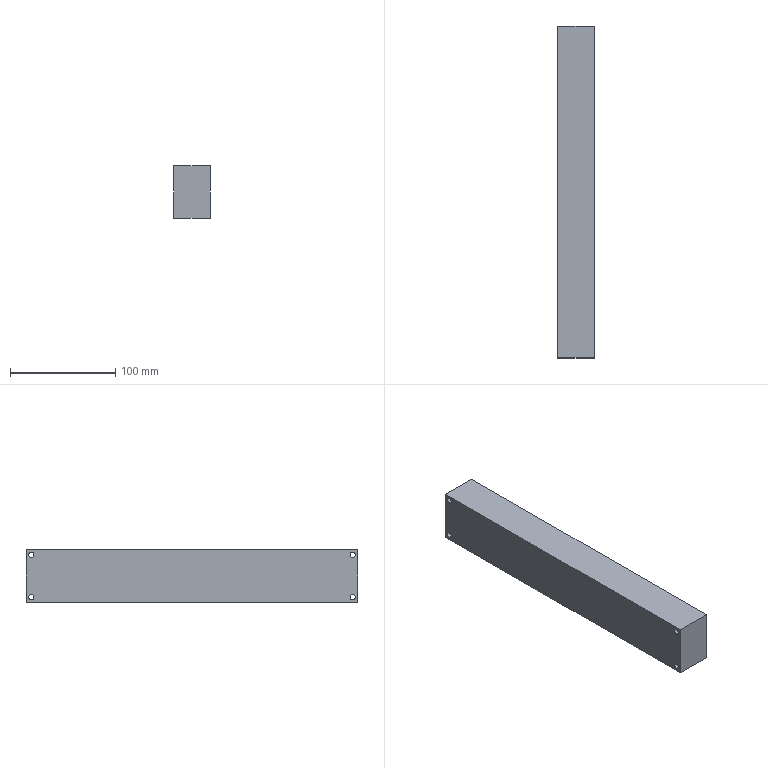Part | SolidWorks | features Extrusion 1, ICE 1 | 1 solid | 14 faces | box 35 x 315 x 50 mm | volume 548501 mm3 | cylinder 8 | plane 6 | commonest cylinder face diameters 5 x8
STEP:
#1=CARTESIAN_POINT('',(35.,5.,2.5));
#2=VERTEX_POINT('',#1);
#3=CARTESIAN_POINT('',(35.,5.,7.5));
#4=VERTEX_POINT('',#3);
#5=CARTESIAN_POINT('',(35.,5.,5.));
#6=DIRECTION('',(-1.,0.,0.));
#7=DIRECTION('',(0.,0.,1.));
#8=AXIS2_PLACEMENT_3D('',#5,#6,#7);
#9=CIRCLE('',#8,2.5);
#10=EDGE_CURVE('',#2,#4,#9,.T.);
#11=ORIENTED_EDGE('',*,*,#10,.F.);
#12=CARTESIAN_POINT('',(0.,5.,2.5));
#13=VERTEX_POINT('',#12);
#14=CARTESIAN_POINT('',(40.,5.,2.5));
#15=DIRECTION('',(-1.,0.,0.));
#16=VECTOR('',#15,1000.);
#17=LINE('',#14,#16);
#18=EDGE_CURVE('',#2,#13,#17,.T.);
#19=ORIENTED_EDGE('',*,*,#18,.T.);
#20=CARTESIAN_POINT('',(0.,5.,7.5));
#21=VERTEX_POINT('',#20);
#22=CARTESIAN_POINT('',(0.,5.,5.));
#23=DIRECTION('',(-1.,0.,0.));
#24=DIRECTION('',(0.,0.,1.));
#25=AXIS2_PLACEMENT_3D('',#22,#23,#24);
#26=CIRCLE('',#25,2.5);
#27=EDGE_CURVE('',#13,#21,#26,.T.);
#28=ORIENTED_EDGE('',*,*,#27,.T.);
#29=CARTESIAN_POINT('',(40.,5.,7.5));
#30=DIRECTION('',(-1.,0.,0.));
#31=VECTOR('',#30,1000.);
#32=LINE('',#29,#31);
#33=EDGE_CURVE('',#4,#21,#32,.T.);
#34=ORIENTED_EDGE('',*,*,#33,.F.);
#35=EDGE_LOOP('',(#11,#19,#28,#34));
#36=FACE_OUTER_BOUND('',#35,.T.);
#37=CARTESIAN_POINT('',(40.,5.,5.));
#38=DIRECTION('',(-1.,0.,0.));
#39=DIRECTION('',(0.,0.,1.));
#40=AXIS2_PLACEMENT_3D('',#37,#38,#39);
#41=CYLINDRICAL_SURFACE('',#40,2.5);
#42=ADVANCED_FACE('',(#36),#41,.F.);
#43=CARTESIAN_POINT('',(35.,5.,42.5));
#44=VERTEX_POINT('',#43);
#45=CARTESIAN_POINT('',(35.,5.,47.5));
#46=VERTEX_POINT('',#45);
#47=CARTESIAN_POINT('',(35.,5.,45.));
#48=DIRECTION('',(-1.,0.,0.));
#49=DIRECTION('',(0.,0.,1.));
#50=AXIS2_PLACEMENT_3D('',#47,#48,#49);
#51=CIRCLE('',#50,2.5);
#52=EDGE_CURVE('',#44,#46,#51,.T.);
#53=ORIENTED_EDGE('',*,*,#52,.F.);
#54=CARTESIAN_POINT('',(0.,5.,42.5));
#55=VERTEX_POINT('',#54);
#56=CARTESIAN_POINT('',(40.,5.,42.5));
#57=DIRECTION('',(-1.,0.,0.));
#58=VECTOR('',#57,1000.);
#59=LINE('',#56,#58);
#60=EDGE_CURVE('',#44,#55,#59,.T.);
#61=ORIENTED_EDGE('',*,*,#60,.T.);
#62=CARTESIAN_POINT('',(0.,5.,47.5));
#63=VERTEX_POINT('',#62);
#64=CARTESIAN_POINT('',(0.,5.,45.));
#65=DIRECTION('',(-1.,0.,0.));
#66=DIRECTION('',(0.,0.,1.));
#67=AXIS2_PLACEMENT_3D('',#64,#65,#66);
#68=CIRCLE('',#67,2.5);
#69=EDGE_CURVE('',#55,#63,#68,.T.);
#70=ORIENTED_EDGE('',*,*,#69,.T.);
#71=CARTESIAN_POINT('',(40.,5.,47.5));
#72=DIRECTION('',(-1.,0.,0.));
#73=VECTOR('',#72,1000.);
#74=LINE('',#71,#73);
#75=EDGE_CURVE('',#46,#63,#74,.T.);
#76=ORIENTED_EDGE('',*,*,#75,.F.);
#77=EDGE_LOOP('',(#53,#61,#70,#76));
#78=FACE_OUTER_BOUND('',#77,.T.);
#79=CARTESIAN_POINT('',(40.,5.,45.));
#80=DIRECTION('',(-1.,0.,0.));
#81=DIRECTION('',(0.,0.,1.));
#82=AXIS2_PLACEMENT_3D('',#79,#80,#81);
#83=CYLINDRICAL_SURFACE('',#82,2.5);
#84=ADVANCED_FACE('',(#78),#83,.F.);
#85=CARTESIAN_POINT('',(35.,310.,2.5));
#86=VERTEX_POINT('',#85);
#87=CARTESIAN_POINT('',(35.,310.,7.5));
#88=VERTEX_POINT('',#87);
#89=CARTESIAN_POINT('',(35.,310.,5.));
#90=DIRECTION('',(-1.,0.,0.));
#91=DIRECTION('',(0.,0.,1.));
#92=AXIS2_PLACEMENT_3D('',#89,#90,#91);
#93=CIRCLE('',#92,2.5);
#94=EDGE_CURVE('',#86,#88,#93,.T.);
#95=ORIENTED_EDGE('',*,*,#94,.F.);
#96=CARTESIAN_POINT('',(0.,310.,2.5));
#97=VERTEX_POINT('',#96);
#98=CARTESIAN_POINT('',(40.,310.,2.5));
#99=DIRECTION('',(-1.,0.,0.));
#100=VECTOR('',#99,1000.);
#101=LINE('',#98,#100);
#102=EDGE_CURVE('',#86,#97,#101,.T.);
#103=ORIENTED_EDGE('',*,*,#102,.T.);
#104=CARTESIAN_POINT('',(0.,310.,7.5));
#105=VERTEX_POINT('',#104);
#106=CARTESIAN_POINT('',(0.,310.,5.));
#107=DIRECTION('',(-1.,0.,0.));
#108=DIRECTION('',(0.,0.,1.));
#109=AXIS2_PLACEMENT_3D('',#106,#107,#108);
#110=CIRCLE('',#109,2.5);
#111=EDGE_CURVE('',#97,#105,#110,.T.);
#112=ORIENTED_EDGE('',*,*,#111,.T.);
#113=CARTESIAN_POINT('',(40.,310.,7.5));
#114=DIRECTION('',(-1.,0.,0.));
#115=VECTOR('',#114,1000.);
#116=LINE('',#113,#115);
#117=EDGE_CURVE('',#88,#105,#116,.T.);
#118=ORIENTED_EDGE('',*,*,#117,.F.);
#119=EDGE_LOOP('',(#95,#103,#112,#118));
#120=FACE_OUTER_BOUND('',#119,.T.);
#121=CARTESIAN_POINT('',(40.,310.,5.));
#122=DIRECTION('',(-1.,0.,0.));
#123=DIRECTION('',(0.,0.,1.));
#124=AXIS2_PLACEMENT_3D('',#121,#122,#123);
#125=CYLINDRICAL_SURFACE('',#124,2.5);
#126=ADVANCED_FACE('',(#120),#125,.F.);
#127=CARTESIAN_POINT('',(35.,310.,42.5));
#128=VERTEX_POINT('',#127);
#129=CARTESIAN_POINT('',(35.,310.,47.5));
#130=VERTEX_POINT('',#129);
#131=CARTESIAN_POINT('',(35.,310.,45.));
#132=DIRECTION('',(-1.,0.,0.));
#133=DIRECTION('',(0.,0.,1.));
#134=AXIS2_PLACEMENT_3D('',#131,#132,#133);
#135=CIRCLE('',#134,2.5);
#136=EDGE_CURVE('',#128,#130,#135,.T.);
#137=ORIENTED_EDGE('',*,*,#136,.F.);
#138=CARTESIAN_POINT('',(0.,310.,42.5));
#139=VERTEX_POINT('',#138);
#140=CARTESIAN_POINT('',(40.,310.,42.5));
#141=DIRECTION('',(-1.,0.,0.));
#142=VECTOR('',#141,1000.);
#143=LINE('',#140,#142);
#144=EDGE_CURVE('',#128,#139,#143,.T.);
#145=ORIENTED_EDGE('',*,*,#144,.T.);
#146=CARTESIAN_POINT('',(0.,310.,47.5));
#147=VERTEX_POINT('',#146);
#148=CARTESIAN_POINT('',(0.,310.,45.));
#149=DIRECTION('',(-1.,0.,0.));
#150=DIRECTION('',(0.,0.,1.));
#151=AXIS2_PLACEMENT_3D('',#148,#149,#150);
#152=CIRCLE('',#151,2.5);
#153=EDGE_CURVE('',#139,#147,#152,.T.);
#154=ORIENTED_EDGE('',*,*,#153,.T.);
#155=CARTESIAN_POINT('',(40.,310.,47.5));
#156=DIRECTION('',(-1.,0.,0.));
#157=VECTOR('',#156,1000.);
#158=LINE('',#155,#157);
#159=EDGE_CURVE('',#130,#147,#158,.T.);
#160=ORIENTED_EDGE('',*,*,#159,.F.);
#161=EDGE_LOOP('',(#137,#145,#154,#160));
#162=FACE_OUTER_BOUND('',#161,.T.);
#163=CARTESIAN_POINT('',(40.,310.,45.));
#164=DIRECTION('',(-1.,0.,0.));
#165=DIRECTION('',(0.,0.,1.));
#166=AXIS2_PLACEMENT_3D('',#163,#164,#165);
#167=CYLINDRICAL_SURFACE('',#166,2.5);
#168=ADVANCED_FACE('',(#162),#167,.F.);
#169=CARTESIAN_POINT('',(0.,5.,5.));
#170=DIRECTION('',(-1.,0.,0.));
#171=DIRECTION('',(0.,0.,1.));
#172=AXIS2_PLACEMENT_3D('',#169,#170,#171);
#173=CIRCLE('',#172,2.5);
#174=EDGE_CURVE('',#21,#13,#173,.T.);
#175=ORIENTED_EDGE('',*,*,#174,.F.);
#176=ORIENTED_EDGE('',*,*,#27,.F.);
#177=EDGE_LOOP('',(#175,#176));
#178=FACE_BOUND('',#177,.T.);
#179=CARTESIAN_POINT('',(0.,5.,45.));
#180=DIRECTION('',(-1.,0.,0.));
#181=DIRECTION('',(0.,0.,1.));
#182=AXIS2_PLACEMENT_3D('',#179,#180,#181);
#183=CIRCLE('',#182,2.5);
#184=EDGE_CURVE('',#63,#55,#183,.T.);
#185=ORIENTED_EDGE('',*,*,#184,.F.);
#186=ORIENTED_EDGE('',*,*,#69,.F.);
#187=EDGE_LOOP('',(#185,#186));
#188=FACE_BOUND('',#187,.T.);
#189=CARTESIAN_POINT('',(0.,310.,5.));
#190=DIRECTION('',(-1.,0.,0.));
#191=DIRECTION('',(0.,0.,1.));
#192=AXIS2_PLACEMENT_3D('',#189,#190,#191);
#193=CIRCLE('',#192,2.5);
#194=EDGE_CURVE('',#105,#97,#193,.T.);
#195=ORIENTED_EDGE('',*,*,#194,.F.);
#196=ORIENTED_EDGE('',*,*,#111,.F.);
#197=EDGE_LOOP('',(#195,#196));
#198=FACE_BOUND('',#197,.T.);
#199=CARTESIAN_POINT('',(0.,310.,45.));
#200=DIRECTION('',(-1.,0.,0.));
#201=DIRECTION('',(0.,0.,1.));
#202=AXIS2_PLACEMENT_3D('',#199,#200,#201);
#203=CIRCLE('',#202,2.5);
#204=EDGE_CURVE('',#147,#139,#203,.T.);
#205=ORIENTED_EDGE('',*,*,#204,.F.);
#206=ORIENTED_EDGE('',*,*,#153,.F.);
#207=EDGE_LOOP('',(#205,#206));
#208=FACE_BOUND('',#207,.T.);
#209=CARTESIAN_POINT('',(0.,315.,0.));
#210=VERTEX_POINT('',#209);
#211=CARTESIAN_POINT('',(0.,0.,0.));
#212=VERTEX_POINT('',#211);
#213=CARTESIAN_POINT('',(0.,0.,0.));
#214=DIRECTION('',(0.,-1.,0.));
#215=VECTOR('',#214,1000.);
#216=LINE('',#213,#215);
#217=EDGE_CURVE('',#210,#212,#216,.T.);
#218=ORIENTED_EDGE('',*,*,#217,.T.);
#219=CARTESIAN_POINT('',(0.,0.,50.));
#220=VERTEX_POINT('',#219);
#221=CARTESIAN_POINT('',(0.,0.,50.));
#222=DIRECTION('',(0.,0.,-1.));
#223=VECTOR('',#222,1000.);
#224=LINE('',#221,#223);
#225=EDGE_CURVE('',#220,#212,#224,.T.);
#226=ORIENTED_EDGE('',*,*,#225,.F.);
#227=CARTESIAN_POINT('',(0.,315.,50.));
#228=VERTEX_POINT('',#227);
#229=CARTESIAN_POINT('',(0.,0.,50.));
#230=DIRECTION('',(0.,-1.,0.));
#231=VECTOR('',#230,1000.);
#232=LINE('',#229,#231);
#233=EDGE_CURVE('',#228,#220,#232,.T.);
#234=ORIENTED_EDGE('',*,*,#233,.F.);
#235=CARTESIAN_POINT('',(0.,315.,50.));
#236=DIRECTION('',(0.,0.,-1.));
#237=VECTOR('',#236,1000.);
#238=LINE('',#235,#237);
#239=EDGE_CURVE('',#228,#210,#238,.T.);
#240=ORIENTED_EDGE('',*,*,#239,.T.);
#241=EDGE_LOOP('',(#218,#226,#234,#240));
#242=FACE_OUTER_BOUND('',#241,.T.);
#243=CARTESIAN_POINT('',(0.,0.,50.));
#244=DIRECTION('',(1.,0.,0.));
#245=DIRECTION('',(0.,0.,-1.));
#246=AXIS2_PLACEMENT_3D('',#243,#244,#245);
#247=PLANE('',#246);
#248=ADVANCED_FACE('',(#178,#188,#198,#208,#242),#247,.F.);
#249=CARTESIAN_POINT('',(35.,0.,0.));
#250=VERTEX_POINT('',#249);
#251=CARTESIAN_POINT('',(0.,0.,0.));
#252=DIRECTION('',(1.,0.,0.));
#253=VECTOR('',#252,1000.);
#254=LINE('',#251,#253);
#255=EDGE_CURVE('',#212,#250,#254,.T.);
#256=ORIENTED_EDGE('',*,*,#255,.T.);
#257=CARTESIAN_POINT('',(35.,0.,50.));
#258=VERTEX_POINT('',#257);
#259=CARTESIAN_POINT('',(35.,0.,50.));
#260=DIRECTION('',(0.,0.,-1.));
#261=VECTOR('',#260,1000.);
#262=LINE('',#259,#261);
#263=EDGE_CURVE('',#258,#250,#262,.T.);
#264=ORIENTED_EDGE('',*,*,#263,.F.);
#265=CARTESIAN_POINT('',(0.,0.,50.));
#266=DIRECTION('',(1.,0.,0.));
#267=VECTOR('',#266,1000.);
#268=LINE('',#265,#267);
#269=EDGE_CURVE('',#220,#258,#268,.T.);
#270=ORIENTED_EDGE('',*,*,#269,.F.);
#271=ORIENTED_EDGE('',*,*,#225,.T.);
#272=EDGE_LOOP('',(#256,#264,#270,#271));
#273=FACE_OUTER_BOUND('',#272,.T.);
#274=CARTESIAN_POINT('',(0.,0.,50.));
#275=DIRECTION('',(0.,1.,0.));
#276=DIRECTION('',(0.,0.,1.));
#277=AXIS2_PLACEMENT_3D('',#274,#275,#276);
#278=PLANE('',#277);
#279=ADVANCED_FACE('',(#273),#278,.F.);
#280=CARTESIAN_POINT('',(35.,5.,5.));
#281=DIRECTION('',(-1.,0.,0.));
#282=DIRECTION('',(0.,0.,1.));
#283=AXIS2_PLACEMENT_3D('',#280,#281,#282);
#284=CIRCLE('',#283,2.5);
#285=EDGE_CURVE('',#4,#2,#284,.T.);
#286=ORIENTED_EDGE('',*,*,#285,.T.);
#287=ORIENTED_EDGE('',*,*,#10,.T.);
#288=EDGE_LOOP('',(#286,#287));
#289=FACE_BOUND('',#288,.T.);
#290=CARTESIAN_POINT('',(35.,5.,45.));
#291=DIRECTION('',(-1.,0.,0.));
#292=DIRECTION('',(0.,0.,1.));
#293=AXIS2_PLACEMENT_3D('',#290,#291,#292);
#294=CIRCLE('',#293,2.5);
#295=EDGE_CURVE('',#46,#44,#294,.T.);
#296=ORIENTED_EDGE('',*,*,#295,.T.);
#297=ORIENTED_EDGE('',*,*,#52,.T.);
#298=EDGE_LOOP('',(#296,#297));
#299=FACE_BOUND('',#298,.T.);
#300=CARTESIAN_POINT('',(35.,310.,5.));
#301=DIRECTION('',(-1.,0.,0.));
#302=DIRECTION('',(0.,0.,1.));
#303=AXIS2_PLACEMENT_3D('',#300,#301,#302);
#304=CIRCLE('',#303,2.5);
#305=EDGE_CURVE('',#88,#86,#304,.T.);
#306=ORIENTED_EDGE('',*,*,#305,.T.);
#307=ORIENTED_EDGE('',*,*,#94,.T.);
#308=EDGE_LOOP('',(#306,#307));
#309=FACE_BOUND('',#308,.T.);
#310=CARTESIAN_POINT('',(35.,310.,45.));
#311=DIRECTION('',(-1.,0.,0.));
#312=DIRECTION('',(0.,0.,1.));
#313=AXIS2_PLACEMENT_3D('',#310,#311,#312);
#314=CIRCLE('',#313,2.5);
#315=EDGE_CURVE('',#130,#128,#314,.T.);
#316=ORIENTED_EDGE('',*,*,#315,.T.);
#317=ORIENTED_EDGE('',*,*,#136,.T.);
#318=EDGE_LOOP('',(#316,#317));
#319=FACE_BOUND('',#318,.T.);
#320=CARTESIAN_POINT('',(35.,315.,0.));
#321=VERTEX_POINT('',#320);
#322=CARTESIAN_POINT('',(35.,0.,0.));
#323=DIRECTION('',(0.,1.,0.));
#324=VECTOR('',#323,1000.);
#325=LINE('',#322,#324);
#326=EDGE_CURVE('',#250,#321,#325,.T.);
#327=ORIENTED_EDGE('',*,*,#326,.T.);
#328=CARTESIAN_POINT('',(35.,315.,50.));
#329=VERTEX_POINT('',#328);
#330=CARTESIAN_POINT('',(35.,315.,50.));
#331=DIRECTION('',(0.,0.,-1.));
#332=VECTOR('',#331,1000.);
#333=LINE('',#330,#332);
#334=EDGE_CURVE('',#329,#321,#333,.T.);
#335=ORIENTED_EDGE('',*,*,#334,.F.);
#336=CARTESIAN_POINT('',(35.,0.,50.));
#337=DIRECTION('',(0.,1.,0.));
#338=VECTOR('',#337,1000.);
#339=LINE('',#336,#338);
#340=EDGE_CURVE('',#258,#329,#339,.T.);
#341=ORIENTED_EDGE('',*,*,#340,.F.);
#342=ORIENTED_EDGE('',*,*,#263,.T.);
#343=EDGE_LOOP('',(#327,#335,#341,#342));
#344=FACE_OUTER_BOUND('',#343,.T.);
#345=CARTESIAN_POINT('',(35.,0.,50.));
#346=DIRECTION('',(-1.,0.,0.));
#347=DIRECTION('',(0.,0.,1.));
#348=AXIS2_PLACEMENT_3D('',#345,#346,#347);
#349=PLANE('',#348);
#350=ADVANCED_FACE('',(#289,#299,#309,#319,#344),#349,.F.);
#351=CARTESIAN_POINT('',(0.,315.,0.));
#352=DIRECTION('',(-1.,0.,0.));
#353=VECTOR('',#352,1000.);
#354=LINE('',#351,#353);
#355=EDGE_CURVE('',#321,#210,#354,.T.);
#356=ORIENTED_EDGE('',*,*,#355,.T.);
#357=ORIENTED_EDGE('',*,*,#239,.F.);
#358=CARTESIAN_POINT('',(0.,315.,50.));
#359=DIRECTION('',(-1.,0.,0.));
#360=VECTOR('',#359,1000.);
#361=LINE('',#358,#360);
#362=EDGE_CURVE('',#329,#228,#361,.T.);
#363=ORIENTED_EDGE('',*,*,#362,.F.);
#364=ORIENTED_EDGE('',*,*,#334,.T.);
#365=EDGE_LOOP('',(#356,#357,#363,#364));
#366=FACE_OUTER_BOUND('',#365,.T.);
#367=CARTESIAN_POINT('',(0.,315.,50.));
#368=DIRECTION('',(0.,-1.,0.));
#369=DIRECTION('',(0.,0.,-1.));
#370=AXIS2_PLACEMENT_3D('',#367,#368,#369);
#371=PLANE('',#370);
#372=ADVANCED_FACE('',(#366),#371,.F.);
#373=ORIENTED_EDGE('',*,*,#233,.T.);
#374=ORIENTED_EDGE('',*,*,#269,.T.);
#375=ORIENTED_EDGE('',*,*,#340,.T.);
#376=ORIENTED_EDGE('',*,*,#362,.T.);
#377=EDGE_LOOP('',(#373,#374,#375,#376));
#378=FACE_OUTER_BOUND('',#377,.T.);
#379=CARTESIAN_POINT('',(0.,315.,50.));
#380=DIRECTION('',(0.,0.,-1.));
#381=DIRECTION('',(-1.,0.,0.));
#382=AXIS2_PLACEMENT_3D('',#379,#380,#381);
#383=PLANE('',#382);
#384=ADVANCED_FACE('',(#378),#383,.F.);
#385=ORIENTED_EDGE('',*,*,#217,.F.);
#386=ORIENTED_EDGE('',*,*,#355,.F.);
#387=ORIENTED_EDGE('',*,*,#326,.F.);
#388=ORIENTED_EDGE('',*,*,#255,.F.);
#389=EDGE_LOOP('',(#385,#386,#387,#388));
#390=FACE_OUTER_BOUND('',#389,.T.);
#391=CARTESIAN_POINT('',(0.,315.,0.));
#392=DIRECTION('',(0.,0.,-1.));
#393=DIRECTION('',(-1.,0.,0.));
#394=AXIS2_PLACEMENT_3D('',#391,#392,#393);
#395=PLANE('',#394);
#396=ADVANCED_FACE('',(#390),#395,.T.);
#397=ORIENTED_EDGE('',*,*,#144,.F.);
#398=ORIENTED_EDGE('',*,*,#315,.F.);
#399=ORIENTED_EDGE('',*,*,#159,.T.);
#400=ORIENTED_EDGE('',*,*,#204,.T.);
#401=EDGE_LOOP('',(#397,#398,#399,#400));
#402=FACE_OUTER_BOUND('',#401,.T.);
#403=CARTESIAN_POINT('',(40.,310.,45.));
#404=DIRECTION('',(-1.,0.,0.));
#405=DIRECTION('',(0.,0.,1.));
#406=AXIS2_PLACEMENT_3D('',#403,#404,#405);
#407=CYLINDRICAL_SURFACE('',#406,2.5);
#408=ADVANCED_FACE('',(#402),#407,.F.);
#409=ORIENTED_EDGE('',*,*,#102,.F.);
#410=ORIENTED_EDGE('',*,*,#305,.F.);
#411=ORIENTED_EDGE('',*,*,#117,.T.);
#412=ORIENTED_EDGE('',*,*,#194,.T.);
#413=EDGE_LOOP('',(#409,#410,#411,#412));
#414=FACE_OUTER_BOUND('',#413,.T.);
#415=CARTESIAN_POINT('',(40.,310.,5.));
#416=DIRECTION('',(-1.,0.,0.));
#417=DIRECTION('',(0.,0.,1.));
#418=AXIS2_PLACEMENT_3D('',#415,#416,#417);
#419=CYLINDRICAL_SURFACE('',#418,2.5);
#420=ADVANCED_FACE('',(#414),#419,.F.);
#421=ORIENTED_EDGE('',*,*,#60,.F.);
#422=ORIENTED_EDGE('',*,*,#295,.F.);
#423=ORIENTED_EDGE('',*,*,#75,.T.);
#424=ORIENTED_EDGE('',*,*,#184,.T.);
#425=EDGE_LOOP('',(#421,#422,#423,#424));
#426=FACE_OUTER_BOUND('',#425,.T.);
#427=CARTESIAN_POINT('',(40.,5.,45.));
#428=DIRECTION('',(-1.,0.,0.));
#429=DIRECTION('',(0.,0.,1.));
#430=AXIS2_PLACEMENT_3D('',#427,#428,#429);
#431=CYLINDRICAL_SURFACE('',#430,2.5);
#432=ADVANCED_FACE('',(#426),#431,.F.);
#433=ORIENTED_EDGE('',*,*,#18,.F.);
#434=ORIENTED_EDGE('',*,*,#285,.F.);
#435=ORIENTED_EDGE('',*,*,#33,.T.);
#436=ORIENTED_EDGE('',*,*,#174,.T.);
#437=EDGE_LOOP('',(#433,#434,#435,#436));
#438=FACE_OUTER_BOUND('',#437,.T.);
#439=CARTESIAN_POINT('',(40.,5.,5.));
#440=DIRECTION('',(-1.,0.,0.));
#441=DIRECTION('',(0.,0.,1.));
#442=AXIS2_PLACEMENT_3D('',#439,#440,#441);
#443=CYLINDRICAL_SURFACE('',#442,2.5);
#444=ADVANCED_FACE('',(#438),#443,.F.);
#445=CLOSED_SHELL('',(#42,#84,#126,#168,#248,#279,#350,#372,#384,#396,#408,#420,#432,#444));
#446=MANIFOLD_SOLID_BREP('',#445);
#447=CARTESIAN_POINT('',(0.,0.,0.));
#448=DIRECTION('',(0.,0.,1.));
#449=DIRECTION('',(1.,0.,0.));
#450=AXIS2_PLACEMENT_3D('',#447,#448,#449);
#451=(LENGTH_UNIT()NAMED_UNIT(*)SI_UNIT(.MILLI.,.METRE.));
#452=UNCERTAINTY_MEASURE_WITH_UNIT(LENGTH_MEASURE(0.00001),#451,'','');
#453=(NAMED_UNIT(*)PLANE_ANGLE_UNIT()SI_UNIT($,.RADIAN.));
#454=(NAMED_UNIT(*)SI_UNIT($,.STERADIAN.)SOLID_ANGLE_UNIT());
#455=(GEOMETRIC_REPRESENTATION_CONTEXT(3)GLOBAL_UNCERTAINTY_ASSIGNED_CONTEXT((#452))GLOBAL_UNIT_ASSIGNED_CONTEXT((#451,#453,#454))REPRESENTATION_CONTEXT('',''));
#456=ADVANCED_BREP_SHAPE_REPRESENTATION('',(#446,#450),#455);